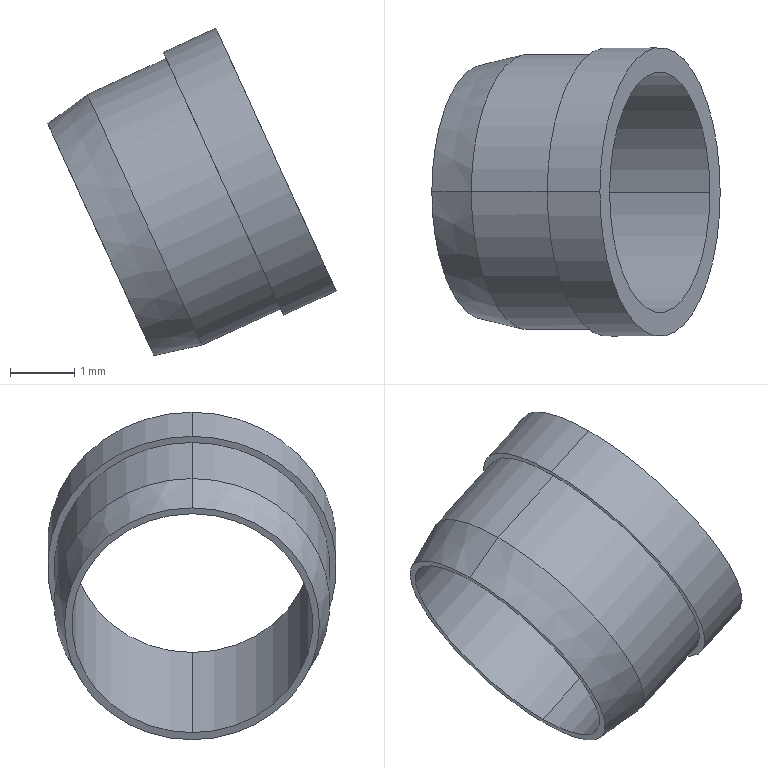Part | STEP file | 2026.6.15-Main Assembly图.sldasm-Part-199 | 1 solid | 11 faces | box 4.491 x 4.5 x 5.1 mm | volume 10.749 mm3 | cylinder 6 | plane 3 | cone 2 | commonest cylinder face diameters 3.75 x2 4.29 x2 4.5 x2
STEP:
#1=CARTESIAN_POINT('',(-1608.049,1442.114,3409.545));
#2=VERTEX_POINT('',#1);
#3=CARTESIAN_POINT('',(-1606.821,1442.114,3410.107));
#4=VERTEX_POINT('',#3);
#5=CARTESIAN_POINT('',(-1583.727,1442.114,3420.681));
#6=DIRECTION('',(0.9092,0.,0.4163));
#7=VECTOR('',#6,1000.);
#8=LINE('',#5,#7);
#9=EDGE_CURVE('',#2,#4,#8,.T.);
#10=ORIENTED_EDGE('',*,*,#9,.T.);
#11=CARTESIAN_POINT('',(-1608.607,1442.114,3414.008));
#12=VERTEX_POINT('',#11);
#13=CARTESIAN_POINT('',(-1607.714,1442.114,3412.058));
#14=DIRECTION('',(0.9092,0.,0.4163));
#15=DIRECTION('',(-0.4163,0.,0.9092));
#16=AXIS2_PLACEMENT_3D('',#13,#14,#15);
#17=CIRCLE('',#16,2.145);
#18=EDGE_CURVE('',#12,#4,#17,.T.);
#19=ORIENTED_EDGE('',*,*,#18,.F.);
#20=CARTESIAN_POINT('',(-1609.835,1442.114,3413.446));
#21=VERTEX_POINT('',#20);
#22=CARTESIAN_POINT('',(-1585.513,1442.114,3424.581));
#23=DIRECTION('',(0.9092,0.,0.4163));
#24=VECTOR('',#23,1000.);
#25=LINE('',#22,#24);
#26=EDGE_CURVE('',#21,#12,#25,.T.);
#27=ORIENTED_EDGE('',*,*,#26,.F.);
#28=CARTESIAN_POINT('',(-1608.942,1442.114,3411.496));
#29=DIRECTION('',(-0.9092,0.,-0.4163));
#30=DIRECTION('',(0.4163,0.,-0.9092));
#31=AXIS2_PLACEMENT_3D('',#28,#29,#30);
#32=CIRCLE('',#31,2.145);
#33=EDGE_CURVE('',#2,#21,#32,.T.);
#34=ORIENTED_EDGE('',*,*,#33,.F.);
#35=EDGE_LOOP('',(#10,#19,#27,#34));
#36=FACE_OUTER_BOUND('',#35,.T.);
#37=CARTESIAN_POINT('',(-1584.62,1442.114,3422.631));
#38=DIRECTION('',(-0.9092,0.,-0.4163));
#39=DIRECTION('',(0.4163,0.,-0.9092));
#40=AXIS2_PLACEMENT_3D('',#37,#38,#39);
#41=CYLINDRICAL_SURFACE('',#40,2.145);
#42=ADVANCED_FACE('',(#36),#41,.T.);
#43=CARTESIAN_POINT('',(-1608.651,1442.114,3414.103));
#44=VERTEX_POINT('',#43);
#45=CARTESIAN_POINT('',(-1606.778,1442.114,3410.012));
#46=VERTEX_POINT('',#45);
#47=CARTESIAN_POINT('',(-1607.714,1442.114,3412.058));
#48=DIRECTION('',(0.9092,0.,0.4163));
#49=DIRECTION('',(-0.4163,0.,0.9092));
#50=AXIS2_PLACEMENT_3D('',#47,#48,#49);
#51=CIRCLE('',#50,2.25);
#52=EDGE_CURVE('',#44,#46,#51,.T.);
#53=ORIENTED_EDGE('',*,*,#52,.F.);
#54=CARTESIAN_POINT('',(-1607.714,1442.114,3412.058));
#55=DIRECTION('',(0.9092,0.,0.4163));
#56=DIRECTION('',(-0.4163,0.,0.9092));
#57=AXIS2_PLACEMENT_3D('',#54,#55,#56);
#58=CIRCLE('',#57,2.25);
#59=EDGE_CURVE('',#46,#44,#58,.T.);
#60=ORIENTED_EDGE('',*,*,#59,.F.);
#61=EDGE_LOOP('',(#53,#60));
#62=FACE_OUTER_BOUND('',#61,.T.);
#63=ORIENTED_EDGE('',*,*,#18,.T.);
#64=CARTESIAN_POINT('',(-1607.714,1442.114,3412.058));
#65=DIRECTION('',(0.9092,0.,0.4163));
#66=DIRECTION('',(-0.4163,0.,0.9092));
#67=AXIS2_PLACEMENT_3D('',#64,#65,#66);
#68=CIRCLE('',#67,2.145);
#69=EDGE_CURVE('',#4,#12,#68,.T.);
#70=ORIENTED_EDGE('',*,*,#69,.T.);
#71=EDGE_LOOP('',(#63,#70));
#72=FACE_BOUND('',#71,.T.);
#73=CARTESIAN_POINT('',(-1607.714,1439.864,3412.058));
#74=DIRECTION('',(-0.9092,0.,-0.4163));
#75=DIRECTION('',(0.,1.,0.));
#76=AXIS2_PLACEMENT_3D('',#73,#74,#75);
#77=PLANE('',#76);
#78=ADVANCED_FACE('',(#62,#72),#77,.T.);
#79=CARTESIAN_POINT('',(-1610.45,1442.114,3412.989));
#80=VERTEX_POINT('',#79);
#81=CARTESIAN_POINT('',(-1609.835,1442.114,3413.446));
#82=DIRECTION('',(0.8028,0.,0.5962));
#83=VECTOR('',#82,1000.);
#84=LINE('',#81,#83);
#85=EDGE_CURVE('',#80,#21,#84,.T.);
#86=ORIENTED_EDGE('',*,*,#85,.F.);
#87=CARTESIAN_POINT('',(-1608.797,1442.114,3409.378));
#88=VERTEX_POINT('',#87);
#89=CARTESIAN_POINT('',(-1609.624,1442.114,3411.183));
#90=DIRECTION('',(-0.9092,0.,-0.4163));
#91=DIRECTION('',(0.4163,0.,-0.9092));
#92=AXIS2_PLACEMENT_3D('',#89,#90,#91);
#93=CIRCLE('',#92,1.986);
#94=EDGE_CURVE('',#88,#80,#93,.T.);
#95=ORIENTED_EDGE('',*,*,#94,.F.);
#96=CARTESIAN_POINT('',(-1608.049,1442.114,3409.545));
#97=DIRECTION('',(0.9759,0.,0.2181));
#98=VECTOR('',#97,1000.);
#99=LINE('',#96,#98);
#100=EDGE_CURVE('',#88,#2,#99,.T.);
#101=ORIENTED_EDGE('',*,*,#100,.T.);
#102=ORIENTED_EDGE('',*,*,#33,.T.);
#103=EDGE_LOOP('',(#86,#95,#101,#102));
#104=FACE_OUTER_BOUND('',#103,.T.);
#105=CARTESIAN_POINT('',(-1608.942,1442.114,3411.496));
#106=DIRECTION('',(0.9092,0.,0.4163));
#107=DIRECTION('',(-0.4163,0.,0.9092));
#108=AXIS2_PLACEMENT_3D('',#105,#106,#107);
#109=CONICAL_SURFACE('',#108,2.145,0.2094);
#110=ADVANCED_FACE('',(#104),#109,.T.);
#111=CARTESIAN_POINT('',(-1605.959,1442.114,3410.387));
#112=VERTEX_POINT('',#111);
#113=CARTESIAN_POINT('',(-1583.683,1442.114,3420.585));
#114=DIRECTION('',(0.9092,0.,0.4163));
#115=VECTOR('',#114,1000.);
#116=LINE('',#113,#115);
#117=EDGE_CURVE('',#46,#112,#116,.T.);
#118=ORIENTED_EDGE('',*,*,#117,.T.);
#119=CARTESIAN_POINT('',(-1607.832,1442.114,3414.478));
#120=VERTEX_POINT('',#119);
#121=CARTESIAN_POINT('',(-1606.896,1442.114,3412.432));
#122=DIRECTION('',(0.9092,0.,0.4163));
#123=DIRECTION('',(-0.4163,0.,0.9092));
#124=AXIS2_PLACEMENT_3D('',#121,#122,#123);
#125=CIRCLE('',#124,2.25);
#126=EDGE_CURVE('',#120,#112,#125,.T.);
#127=ORIENTED_EDGE('',*,*,#126,.F.);
#128=CARTESIAN_POINT('',(-1585.556,1442.114,3424.677));
#129=DIRECTION('',(0.9092,0.,0.4163));
#130=VECTOR('',#129,1000.);
#131=LINE('',#128,#130);
#132=EDGE_CURVE('',#44,#120,#131,.T.);
#133=ORIENTED_EDGE('',*,*,#132,.F.);
#134=ORIENTED_EDGE('',*,*,#52,.T.);
#135=EDGE_LOOP('',(#118,#127,#133,#134));
#136=FACE_OUTER_BOUND('',#135,.T.);
#137=CARTESIAN_POINT('',(-1584.62,1442.114,3422.631));
#138=DIRECTION('',(-0.9092,0.,-0.4163));
#139=DIRECTION('',(0.4163,0.,-0.9092));
#140=AXIS2_PLACEMENT_3D('',#137,#138,#139);
#141=CYLINDRICAL_SURFACE('',#140,2.25);
#142=ADVANCED_FACE('',(#136),#141,.T.);
#143=ORIENTED_EDGE('',*,*,#94,.T.);
#144=CARTESIAN_POINT('',(-1609.624,1442.114,3411.183));
#145=DIRECTION('',(-0.9092,0.,-0.4163));
#146=DIRECTION('',(0.4163,0.,-0.9092));
#147=AXIS2_PLACEMENT_3D('',#144,#145,#146);
#148=CIRCLE('',#147,1.986);
#149=EDGE_CURVE('',#80,#88,#148,.T.);
#150=ORIENTED_EDGE('',*,*,#149,.T.);
#151=EDGE_LOOP('',(#143,#150));
#152=FACE_OUTER_BOUND('',#151,.T.);
#153=CARTESIAN_POINT('',(-1610.408,1442.111,3412.898));
#154=VERTEX_POINT('',#153);
#155=CARTESIAN_POINT('',(-1608.847,1442.111,3409.488));
#156=VERTEX_POINT('',#155);
#157=CARTESIAN_POINT('',(-1609.628,1442.111,3411.193));
#158=DIRECTION('',(0.9092,0.,0.4163));
#159=DIRECTION('',(-0.4163,0.,0.9092));
#160=AXIS2_PLACEMENT_3D('',#157,#158,#159);
#161=CIRCLE('',#160,1.875);
#162=EDGE_CURVE('',#154,#156,#161,.T.);
#163=ORIENTED_EDGE('',*,*,#162,.T.);
#164=CARTESIAN_POINT('',(-1609.628,1442.111,3411.193));
#165=DIRECTION('',(0.9092,0.,0.4163));
#166=DIRECTION('',(-0.4163,0.,0.9092));
#167=AXIS2_PLACEMENT_3D('',#164,#165,#166);
#168=CIRCLE('',#167,1.875);
#169=EDGE_CURVE('',#156,#154,#168,.T.);
#170=ORIENTED_EDGE('',*,*,#169,.T.);
#171=EDGE_LOOP('',(#163,#170));
#172=FACE_BOUND('',#171,.T.);
#173=CARTESIAN_POINT('',(-1609.624,1440.129,3411.183));
#174=DIRECTION('',(-0.9092,0.,-0.4163));
#175=DIRECTION('',(0.,1.,0.));
#176=AXIS2_PLACEMENT_3D('',#173,#174,#175);
#177=PLANE('',#176);
#178=ADVANCED_FACE('',(#152,#172),#177,.T.);
#179=ORIENTED_EDGE('',*,*,#126,.T.);
#180=CARTESIAN_POINT('',(-1606.896,1442.114,3412.432));
#181=DIRECTION('',(0.9092,0.,0.4163));
#182=DIRECTION('',(-0.4163,0.,0.9092));
#183=AXIS2_PLACEMENT_3D('',#180,#181,#182);
#184=CIRCLE('',#183,2.25);
#185=EDGE_CURVE('',#112,#120,#184,.T.);
#186=ORIENTED_EDGE('',*,*,#185,.T.);
#187=EDGE_LOOP('',(#179,#186));
#188=FACE_OUTER_BOUND('',#187,.T.);
#189=CARTESIAN_POINT('',(-1607.681,1442.111,3414.147));
#190=VERTEX_POINT('',#189);
#191=CARTESIAN_POINT('',(-1606.12,1442.111,3410.737));
#192=VERTEX_POINT('',#191);
#193=CARTESIAN_POINT('',(-1606.9,1442.111,3412.442));
#194=DIRECTION('',(-0.9092,0.,-0.4163));
#195=DIRECTION('',(-0.4163,0.,0.9092));
#196=AXIS2_PLACEMENT_3D('',#193,#194,#195);
#197=CIRCLE('',#196,1.875);
#198=EDGE_CURVE('',#190,#192,#197,.T.);
#199=ORIENTED_EDGE('',*,*,#198,.T.);
#200=CARTESIAN_POINT('',(-1606.9,1442.111,3412.442));
#201=DIRECTION('',(-0.9092,0.,-0.4163));
#202=DIRECTION('',(-0.4163,0.,0.9092));
#203=AXIS2_PLACEMENT_3D('',#200,#201,#202);
#204=CIRCLE('',#203,1.875);
#205=EDGE_CURVE('',#192,#190,#204,.T.);
#206=ORIENTED_EDGE('',*,*,#205,.T.);
#207=EDGE_LOOP('',(#199,#206));
#208=FACE_BOUND('',#207,.T.);
#209=CARTESIAN_POINT('',(-1606.896,1442.114,3412.432));
#210=DIRECTION('',(0.9092,0.,0.4163));
#211=DIRECTION('',(-0.4163,0.,0.9092));
#212=AXIS2_PLACEMENT_3D('',#209,#210,#211);
#213=PLANE('',#212);
#214=ADVANCED_FACE('',(#188,#208),#213,.T.);
#215=CARTESIAN_POINT('',(-1637.761,1442.111,3396.251));
#216=DIRECTION('',(0.9092,0.,0.4163));
#217=VECTOR('',#216,1000.);
#218=LINE('',#215,#217);
#219=EDGE_CURVE('',#156,#192,#218,.T.);
#220=ORIENTED_EDGE('',*,*,#219,.T.);
#221=ORIENTED_EDGE('',*,*,#198,.F.);
#222=CARTESIAN_POINT('',(-1639.322,1442.111,3399.66));
#223=DIRECTION('',(0.9092,0.,0.4163));
#224=VECTOR('',#223,1000.);
#225=LINE('',#222,#224);
#226=EDGE_CURVE('',#154,#190,#225,.T.);
#227=ORIENTED_EDGE('',*,*,#226,.F.);
#228=ORIENTED_EDGE('',*,*,#169,.F.);
#229=EDGE_LOOP('',(#220,#221,#227,#228));
#230=FACE_OUTER_BOUND('',#229,.T.);
#231=CARTESIAN_POINT('',(-1638.542,1442.111,3397.955));
#232=DIRECTION('',(-0.9092,0.,-0.4163));
#233=DIRECTION('',(0.4163,0.,-0.9092));
#234=AXIS2_PLACEMENT_3D('',#231,#232,#233);
#235=CYLINDRICAL_SURFACE('',#234,1.875);
#236=ADVANCED_FACE('',(#230),#235,.F.);
#237=ORIENTED_EDGE('',*,*,#69,.F.);
#238=ORIENTED_EDGE('',*,*,#9,.F.);
#239=CARTESIAN_POINT('',(-1608.942,1442.114,3411.496));
#240=DIRECTION('',(-0.9092,0.,-0.4163));
#241=DIRECTION('',(0.4163,0.,-0.9092));
#242=AXIS2_PLACEMENT_3D('',#239,#240,#241);
#243=CIRCLE('',#242,2.145);
#244=EDGE_CURVE('',#21,#2,#243,.T.);
#245=ORIENTED_EDGE('',*,*,#244,.F.);
#246=ORIENTED_EDGE('',*,*,#26,.T.);
#247=EDGE_LOOP('',(#237,#238,#245,#246));
#248=FACE_OUTER_BOUND('',#247,.T.);
#249=CARTESIAN_POINT('',(-1584.62,1442.114,3422.631));
#250=DIRECTION('',(-0.9092,0.,-0.4163));
#251=DIRECTION('',(0.4163,0.,-0.9092));
#252=AXIS2_PLACEMENT_3D('',#249,#250,#251);
#253=CYLINDRICAL_SURFACE('',#252,2.145);
#254=ADVANCED_FACE('',(#248),#253,.T.);
#255=ORIENTED_EDGE('',*,*,#149,.F.);
#256=ORIENTED_EDGE('',*,*,#85,.T.);
#257=ORIENTED_EDGE('',*,*,#244,.T.);
#258=ORIENTED_EDGE('',*,*,#100,.F.);
#259=EDGE_LOOP('',(#255,#256,#257,#258));
#260=FACE_OUTER_BOUND('',#259,.T.);
#261=CARTESIAN_POINT('',(-1608.942,1442.114,3411.496));
#262=DIRECTION('',(0.9092,0.,0.4163));
#263=DIRECTION('',(-0.4163,0.,0.9092));
#264=AXIS2_PLACEMENT_3D('',#261,#262,#263);
#265=CONICAL_SURFACE('',#264,2.145,0.2094);
#266=ADVANCED_FACE('',(#260),#265,.T.);
#267=ORIENTED_EDGE('',*,*,#185,.F.);
#268=ORIENTED_EDGE('',*,*,#117,.F.);
#269=ORIENTED_EDGE('',*,*,#59,.T.);
#270=ORIENTED_EDGE('',*,*,#132,.T.);
#271=EDGE_LOOP('',(#267,#268,#269,#270));
#272=FACE_OUTER_BOUND('',#271,.T.);
#273=CARTESIAN_POINT('',(-1584.62,1442.114,3422.631));
#274=DIRECTION('',(-0.9092,0.,-0.4163));
#275=DIRECTION('',(0.4163,0.,-0.9092));
#276=AXIS2_PLACEMENT_3D('',#273,#274,#275);
#277=CYLINDRICAL_SURFACE('',#276,2.25);
#278=ADVANCED_FACE('',(#272),#277,.T.);
#279=ORIENTED_EDGE('',*,*,#205,.F.);
#280=ORIENTED_EDGE('',*,*,#219,.F.);
#281=ORIENTED_EDGE('',*,*,#162,.F.);
#282=ORIENTED_EDGE('',*,*,#226,.T.);
#283=EDGE_LOOP('',(#279,#280,#281,#282));
#284=FACE_OUTER_BOUND('',#283,.T.);
#285=CARTESIAN_POINT('',(-1638.542,1442.111,3397.955));
#286=DIRECTION('',(-0.9092,0.,-0.4163));
#287=DIRECTION('',(0.4163,0.,-0.9092));
#288=AXIS2_PLACEMENT_3D('',#285,#286,#287);
#289=CYLINDRICAL_SURFACE('',#288,1.875);
#290=ADVANCED_FACE('',(#284),#289,.F.);
#291=CLOSED_SHELL('',(#42,#78,#110,#142,#178,#214,#236,#254,#266,#278,#290));
#292=MANIFOLD_SOLID_BREP('',#291);
#293=CARTESIAN_POINT('',(0.,0.,0.));
#294=DIRECTION('',(0.,0.,1.));
#295=DIRECTION('',(1.,0.,0.));
#296=AXIS2_PLACEMENT_3D('',#293,#294,#295);
#297=(LENGTH_UNIT()NAMED_UNIT(*)SI_UNIT(.MILLI.,.METRE.));
#298=UNCERTAINTY_MEASURE_WITH_UNIT(LENGTH_MEASURE(0.00001),#297,'','');
#299=(NAMED_UNIT(*)PLANE_ANGLE_UNIT()SI_UNIT($,.RADIAN.));
#300=(NAMED_UNIT(*)SI_UNIT($,.STERADIAN.)SOLID_ANGLE_UNIT());
#301=(GEOMETRIC_REPRESENTATION_CONTEXT(3)GLOBAL_UNCERTAINTY_ASSIGNED_CONTEXT((#298))GLOBAL_UNIT_ASSIGNED_CONTEXT((#297,#299,#300))REPRESENTATION_CONTEXT('',''));
#302=ADVANCED_BREP_SHAPE_REPRESENTATION('',(#292,#296),#301);